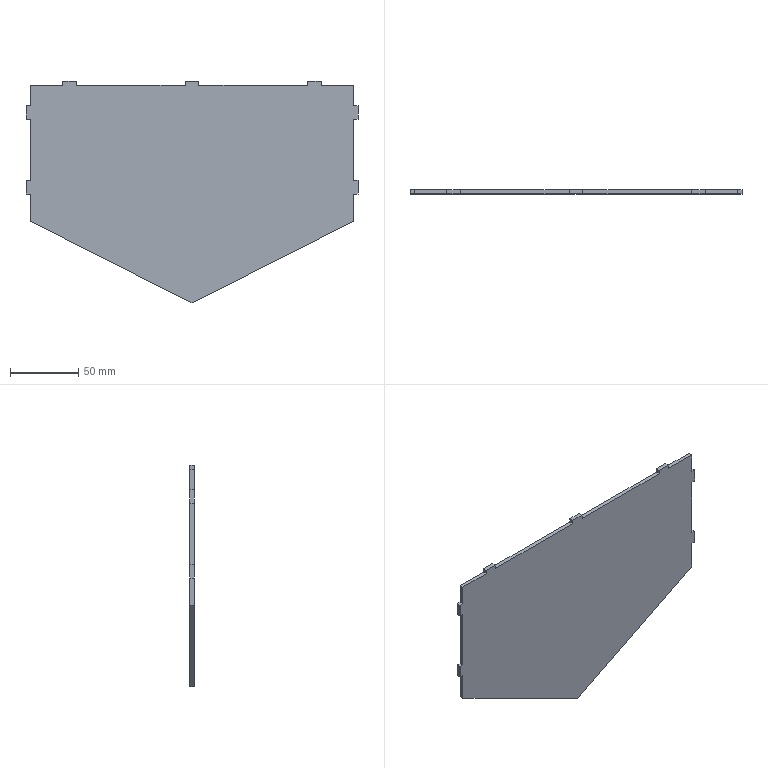Part | SolidWorks | features Extrusion 1, ICE 1 | 1 solid | 35 faces | box 244 x 3 x 163 mm | volume 93450 mm3 | plane 35
STEP:
#1=CARTESIAN_POINT('',(5.,3.,50.));
#2=VERTEX_POINT('',#1);
#3=CARTESIAN_POINT('',(85.,3.,50.));
#4=VERTEX_POINT('',#3);
#5=CARTESIAN_POINT('',(-119.,3.,50.));
#6=DIRECTION('',(1.,0.,0.));
#7=VECTOR('',#6,1000.);
#8=LINE('',#5,#7);
#9=EDGE_CURVE('',#2,#4,#8,.T.);
#10=ORIENTED_EDGE('',*,*,#9,.F.);
#11=CARTESIAN_POINT('',(5.,0.,50.));
#12=VERTEX_POINT('',#11);
#13=CARTESIAN_POINT('',(5.,-10.44,50.));
#14=DIRECTION('',(0.,1.,0.));
#15=VECTOR('',#14,1000.);
#16=LINE('',#13,#15);
#17=EDGE_CURVE('',#12,#2,#16,.T.);
#18=ORIENTED_EDGE('',*,*,#17,.F.);
#19=CARTESIAN_POINT('',(85.,0.,50.));
#20=VERTEX_POINT('',#19);
#21=CARTESIAN_POINT('',(-119.,0.,50.));
#22=DIRECTION('',(1.,0.,0.));
#23=VECTOR('',#22,1000.);
#24=LINE('',#21,#23);
#25=EDGE_CURVE('',#12,#20,#24,.T.);
#26=ORIENTED_EDGE('',*,*,#25,.T.);
#27=CARTESIAN_POINT('',(85.,-10.44,50.));
#28=DIRECTION('',(0.,1.,0.));
#29=VECTOR('',#28,1000.);
#30=LINE('',#27,#29);
#31=EDGE_CURVE('',#20,#4,#30,.T.);
#32=ORIENTED_EDGE('',*,*,#31,.T.);
#33=EDGE_LOOP('',(#10,#18,#26,#32));
#34=FACE_OUTER_BOUND('',#33,.T.);
#35=CARTESIAN_POINT('',(-119.,3.,50.));
#36=DIRECTION('',(0.,0.,-1.));
#37=DIRECTION('',(-1.,0.,0.));
#38=AXIS2_PLACEMENT_3D('',#35,#36,#37);
#39=PLANE('',#38);
#40=ADVANCED_FACE('',(#34),#39,.F.);
#41=CARTESIAN_POINT('',(-85.,0.,50.));
#42=VERTEX_POINT('',#41);
#43=CARTESIAN_POINT('',(-5.,0.,50.));
#44=VERTEX_POINT('',#43);
#45=CARTESIAN_POINT('',(-119.,0.,50.));
#46=DIRECTION('',(1.,0.,0.));
#47=VECTOR('',#46,1000.);
#48=LINE('',#45,#47);
#49=EDGE_CURVE('',#42,#44,#48,.T.);
#50=ORIENTED_EDGE('',*,*,#49,.T.);
#51=CARTESIAN_POINT('',(-5.,3.,50.));
#52=VERTEX_POINT('',#51);
#53=CARTESIAN_POINT('',(-5.,-10.44,50.));
#54=DIRECTION('',(0.,1.,0.));
#55=VECTOR('',#54,1000.);
#56=LINE('',#53,#55);
#57=EDGE_CURVE('',#44,#52,#56,.T.);
#58=ORIENTED_EDGE('',*,*,#57,.T.);
#59=CARTESIAN_POINT('',(-85.,3.,50.));
#60=VERTEX_POINT('',#59);
#61=CARTESIAN_POINT('',(-119.,3.,50.));
#62=DIRECTION('',(1.,0.,0.));
#63=VECTOR('',#62,1000.);
#64=LINE('',#61,#63);
#65=EDGE_CURVE('',#60,#52,#64,.T.);
#66=ORIENTED_EDGE('',*,*,#65,.F.);
#67=CARTESIAN_POINT('',(-85.,-10.44,50.));
#68=DIRECTION('',(0.,1.,0.));
#69=VECTOR('',#68,1000.);
#70=LINE('',#67,#69);
#71=EDGE_CURVE('',#42,#60,#70,.T.);
#72=ORIENTED_EDGE('',*,*,#71,.F.);
#73=EDGE_LOOP('',(#50,#58,#66,#72));
#74=FACE_OUTER_BOUND('',#73,.T.);
#75=CARTESIAN_POINT('',(-119.,3.,50.));
#76=DIRECTION('',(0.,0.,-1.));
#77=DIRECTION('',(-1.,0.,0.));
#78=AXIS2_PLACEMENT_3D('',#75,#76,#77);
#79=PLANE('',#78);
#80=ADVANCED_FACE('',(#74),#79,.F.);
#81=CARTESIAN_POINT('',(95.,0.,50.));
#82=VERTEX_POINT('',#81);
#83=CARTESIAN_POINT('',(95.,3.,50.));
#84=VERTEX_POINT('',#83);
#85=CARTESIAN_POINT('',(95.,-10.44,50.));
#86=DIRECTION('',(0.,1.,0.));
#87=VECTOR('',#86,1000.);
#88=LINE('',#85,#87);
#89=EDGE_CURVE('',#82,#84,#88,.T.);
#90=ORIENTED_EDGE('',*,*,#89,.F.);
#91=CARTESIAN_POINT('',(119.,0.,50.));
#92=VERTEX_POINT('',#91);
#93=CARTESIAN_POINT('',(-119.,0.,50.));
#94=DIRECTION('',(1.,0.,0.));
#95=VECTOR('',#94,1000.);
#96=LINE('',#93,#95);
#97=EDGE_CURVE('',#82,#92,#96,.T.);
#98=ORIENTED_EDGE('',*,*,#97,.T.);
#99=CARTESIAN_POINT('',(119.,3.,50.));
#100=VERTEX_POINT('',#99);
#101=CARTESIAN_POINT('',(119.,3.,50.));
#102=DIRECTION('',(0.,-1.,0.));
#103=VECTOR('',#102,1000.);
#104=LINE('',#101,#103);
#105=EDGE_CURVE('',#100,#92,#104,.T.);
#106=ORIENTED_EDGE('',*,*,#105,.F.);
#107=CARTESIAN_POINT('',(-119.,3.,50.));
#108=DIRECTION('',(1.,0.,0.));
#109=VECTOR('',#108,1000.);
#110=LINE('',#107,#109);
#111=EDGE_CURVE('',#84,#100,#110,.T.);
#112=ORIENTED_EDGE('',*,*,#111,.F.);
#113=EDGE_LOOP('',(#90,#98,#106,#112));
#114=FACE_OUTER_BOUND('',#113,.T.);
#115=CARTESIAN_POINT('',(-119.,3.,50.));
#116=DIRECTION('',(0.,0.,-1.));
#117=DIRECTION('',(-1.,0.,0.));
#118=AXIS2_PLACEMENT_3D('',#115,#116,#117);
#119=PLANE('',#118);
#120=ADVANCED_FACE('',(#114),#119,.F.);
#121=CARTESIAN_POINT('',(-119.,0.,-50.));
#122=VERTEX_POINT('',#121);
#123=CARTESIAN_POINT('',(-119.,0.,-30.));
#124=VERTEX_POINT('',#123);
#125=CARTESIAN_POINT('',(-119.,0.,50.));
#126=DIRECTION('',(0.,0.,1.));
#127=VECTOR('',#126,1000.);
#128=LINE('',#125,#127);
#129=EDGE_CURVE('',#122,#124,#128,.T.);
#130=ORIENTED_EDGE('',*,*,#129,.T.);
#131=CARTESIAN_POINT('',(-119.,3.,-30.));
#132=VERTEX_POINT('',#131);
#133=CARTESIAN_POINT('',(-119.,-10.44,-30.));
#134=DIRECTION('',(0.,1.,0.));
#135=VECTOR('',#134,1000.);
#136=LINE('',#133,#135);
#137=EDGE_CURVE('',#124,#132,#136,.T.);
#138=ORIENTED_EDGE('',*,*,#137,.T.);
#139=CARTESIAN_POINT('',(-119.,3.,-50.));
#140=VERTEX_POINT('',#139);
#141=CARTESIAN_POINT('',(-119.,3.,50.));
#142=DIRECTION('',(0.,0.,1.));
#143=VECTOR('',#142,1000.);
#144=LINE('',#141,#143);
#145=EDGE_CURVE('',#140,#132,#144,.T.);
#146=ORIENTED_EDGE('',*,*,#145,.F.);
#147=CARTESIAN_POINT('',(-119.,3.,-50.));
#148=DIRECTION('',(0.,-1.,0.));
#149=VECTOR('',#148,1000.);
#150=LINE('',#147,#149);
#151=EDGE_CURVE('',#140,#122,#150,.T.);
#152=ORIENTED_EDGE('',*,*,#151,.T.);
#153=EDGE_LOOP('',(#130,#138,#146,#152));
#154=FACE_OUTER_BOUND('',#153,.T.);
#155=CARTESIAN_POINT('',(-119.,3.,50.));
#156=DIRECTION('',(1.,0.,0.));
#157=DIRECTION('',(0.,0.,-1.));
#158=AXIS2_PLACEMENT_3D('',#155,#156,#157);
#159=PLANE('',#158);
#160=ADVANCED_FACE('',(#154),#159,.F.);
#161=CARTESIAN_POINT('',(-119.,0.,35.));
#162=VERTEX_POINT('',#161);
#163=CARTESIAN_POINT('',(-119.,3.,35.));
#164=VERTEX_POINT('',#163);
#165=CARTESIAN_POINT('',(-119.,-10.44,35.));
#166=DIRECTION('',(0.,1.,0.));
#167=VECTOR('',#166,1000.);
#168=LINE('',#165,#167);
#169=EDGE_CURVE('',#162,#164,#168,.T.);
#170=ORIENTED_EDGE('',*,*,#169,.F.);
#171=CARTESIAN_POINT('',(-119.,0.,50.));
#172=VERTEX_POINT('',#171);
#173=CARTESIAN_POINT('',(-119.,0.,50.));
#174=DIRECTION('',(0.,0.,1.));
#175=VECTOR('',#174,1000.);
#176=LINE('',#173,#175);
#177=EDGE_CURVE('',#162,#172,#176,.T.);
#178=ORIENTED_EDGE('',*,*,#177,.T.);
#179=CARTESIAN_POINT('',(-119.,3.,50.));
#180=VERTEX_POINT('',#179);
#181=CARTESIAN_POINT('',(-119.,3.,50.));
#182=DIRECTION('',(0.,-1.,0.));
#183=VECTOR('',#182,1000.);
#184=LINE('',#181,#183);
#185=EDGE_CURVE('',#180,#172,#184,.T.);
#186=ORIENTED_EDGE('',*,*,#185,.F.);
#187=CARTESIAN_POINT('',(-119.,3.,50.));
#188=DIRECTION('',(0.,0.,1.));
#189=VECTOR('',#188,1000.);
#190=LINE('',#187,#189);
#191=EDGE_CURVE('',#164,#180,#190,.T.);
#192=ORIENTED_EDGE('',*,*,#191,.F.);
#193=EDGE_LOOP('',(#170,#178,#186,#192));
#194=FACE_OUTER_BOUND('',#193,.T.);
#195=CARTESIAN_POINT('',(-119.,3.,50.));
#196=DIRECTION('',(1.,0.,0.));
#197=DIRECTION('',(0.,0.,-1.));
#198=AXIS2_PLACEMENT_3D('',#195,#196,#197);
#199=PLANE('',#198);
#200=ADVANCED_FACE('',(#194),#199,.F.);
#201=CARTESIAN_POINT('',(119.,3.,25.));
#202=VERTEX_POINT('',#201);
#203=CARTESIAN_POINT('',(119.,3.,-20.));
#204=VERTEX_POINT('',#203);
#205=CARTESIAN_POINT('',(119.,3.,50.));
#206=DIRECTION('',(0.,0.,-1.));
#207=VECTOR('',#206,1000.);
#208=LINE('',#205,#207);
#209=EDGE_CURVE('',#202,#204,#208,.T.);
#210=ORIENTED_EDGE('',*,*,#209,.F.);
#211=CARTESIAN_POINT('',(119.,0.,25.));
#212=VERTEX_POINT('',#211);
#213=CARTESIAN_POINT('',(119.,-10.44,25.));
#214=DIRECTION('',(0.,1.,0.));
#215=VECTOR('',#214,1000.);
#216=LINE('',#213,#215);
#217=EDGE_CURVE('',#212,#202,#216,.T.);
#218=ORIENTED_EDGE('',*,*,#217,.F.);
#219=CARTESIAN_POINT('',(119.,0.,-20.));
#220=VERTEX_POINT('',#219);
#221=CARTESIAN_POINT('',(119.,0.,50.));
#222=DIRECTION('',(0.,0.,-1.));
#223=VECTOR('',#222,1000.);
#224=LINE('',#221,#223);
#225=EDGE_CURVE('',#212,#220,#224,.T.);
#226=ORIENTED_EDGE('',*,*,#225,.T.);
#227=CARTESIAN_POINT('',(119.,-10.44,-20.));
#228=DIRECTION('',(0.,1.,0.));
#229=VECTOR('',#228,1000.);
#230=LINE('',#227,#229);
#231=EDGE_CURVE('',#220,#204,#230,.T.);
#232=ORIENTED_EDGE('',*,*,#231,.T.);
#233=EDGE_LOOP('',(#210,#218,#226,#232));
#234=FACE_OUTER_BOUND('',#233,.T.);
#235=CARTESIAN_POINT('',(119.,3.,50.));
#236=DIRECTION('',(-1.,0.,0.));
#237=DIRECTION('',(0.,0.,1.));
#238=AXIS2_PLACEMENT_3D('',#235,#236,#237);
#239=PLANE('',#238);
#240=ADVANCED_FACE('',(#234),#239,.F.);
#241=CARTESIAN_POINT('',(119.,0.,-30.));
#242=VERTEX_POINT('',#241);
#243=CARTESIAN_POINT('',(119.,3.,-30.));
#244=VERTEX_POINT('',#243);
#245=CARTESIAN_POINT('',(119.,-10.44,-30.));
#246=DIRECTION('',(0.,1.,0.));
#247=VECTOR('',#246,1000.);
#248=LINE('',#245,#247);
#249=EDGE_CURVE('',#242,#244,#248,.T.);
#250=ORIENTED_EDGE('',*,*,#249,.F.);
#251=CARTESIAN_POINT('',(119.,0.,-50.));
#252=VERTEX_POINT('',#251);
#253=CARTESIAN_POINT('',(119.,0.,50.));
#254=DIRECTION('',(0.,0.,-1.));
#255=VECTOR('',#254,1000.);
#256=LINE('',#253,#255);
#257=EDGE_CURVE('',#242,#252,#256,.T.);
#258=ORIENTED_EDGE('',*,*,#257,.T.);
#259=CARTESIAN_POINT('',(119.,3.,-50.));
#260=VERTEX_POINT('',#259);
#261=CARTESIAN_POINT('',(119.,3.,-50.));
#262=DIRECTION('',(0.,-1.,0.));
#263=VECTOR('',#262,1000.);
#264=LINE('',#261,#263);
#265=EDGE_CURVE('',#260,#252,#264,.T.);
#266=ORIENTED_EDGE('',*,*,#265,.F.);
#267=CARTESIAN_POINT('',(119.,3.,50.));
#268=DIRECTION('',(0.,0.,-1.));
#269=VECTOR('',#268,1000.);
#270=LINE('',#267,#269);
#271=EDGE_CURVE('',#244,#260,#270,.T.);
#272=ORIENTED_EDGE('',*,*,#271,.F.);
#273=EDGE_LOOP('',(#250,#258,#266,#272));
#274=FACE_OUTER_BOUND('',#273,.T.);
#275=CARTESIAN_POINT('',(119.,3.,50.));
#276=DIRECTION('',(-1.,0.,0.));
#277=DIRECTION('',(0.,0.,1.));
#278=AXIS2_PLACEMENT_3D('',#275,#276,#277);
#279=PLANE('',#278);
#280=ADVANCED_FACE('',(#274),#279,.F.);
#281=CARTESIAN_POINT('',(0.,0.,-110.));
#282=VERTEX_POINT('',#281);
#283=CARTESIAN_POINT('',(0.,0.,-110.));
#284=DIRECTION('',(-0.8929,0.,-0.4502));
#285=VECTOR('',#284,1000.);
#286=LINE('',#283,#285);
#287=EDGE_CURVE('',#252,#282,#286,.T.);
#288=ORIENTED_EDGE('',*,*,#287,.T.);
#289=CARTESIAN_POINT('',(0.,3.,-110.));
#290=VERTEX_POINT('',#289);
#291=CARTESIAN_POINT('',(0.,3.,-110.));
#292=DIRECTION('',(0.,-1.,0.));
#293=VECTOR('',#292,1000.);
#294=LINE('',#291,#293);
#295=EDGE_CURVE('',#290,#282,#294,.T.);
#296=ORIENTED_EDGE('',*,*,#295,.F.);
#297=CARTESIAN_POINT('',(0.,3.,-110.));
#298=DIRECTION('',(-0.8929,0.,-0.4502));
#299=VECTOR('',#298,1000.);
#300=LINE('',#297,#299);
#301=EDGE_CURVE('',#260,#290,#300,.T.);
#302=ORIENTED_EDGE('',*,*,#301,.F.);
#303=ORIENTED_EDGE('',*,*,#265,.T.);
#304=EDGE_LOOP('',(#288,#296,#302,#303));
#305=FACE_OUTER_BOUND('',#304,.T.);
#306=CARTESIAN_POINT('',(0.,3.,-110.));
#307=DIRECTION('',(-0.4502,0.,0.8929));
#308=DIRECTION('',(0.8929,0.,0.4502));
#309=AXIS2_PLACEMENT_3D('',#306,#307,#308);
#310=PLANE('',#309);
#311=ADVANCED_FACE('',(#305),#310,.F.);
#312=CARTESIAN_POINT('',(-119.,0.,-50.));
#313=DIRECTION('',(-0.8929,0.,0.4502));
#314=VECTOR('',#313,1000.);
#315=LINE('',#312,#314);
#316=EDGE_CURVE('',#282,#122,#315,.T.);
#317=ORIENTED_EDGE('',*,*,#316,.T.);
#318=ORIENTED_EDGE('',*,*,#151,.F.);
#319=CARTESIAN_POINT('',(-119.,3.,-50.));
#320=DIRECTION('',(-0.8929,0.,0.4502));
#321=VECTOR('',#320,1000.);
#322=LINE('',#319,#321);
#323=EDGE_CURVE('',#290,#140,#322,.T.);
#324=ORIENTED_EDGE('',*,*,#323,.F.);
#325=ORIENTED_EDGE('',*,*,#295,.T.);
#326=EDGE_LOOP('',(#317,#318,#324,#325));
#327=FACE_OUTER_BOUND('',#326,.T.);
#328=CARTESIAN_POINT('',(-119.,3.,-50.));
#329=DIRECTION('',(0.4502,0.,0.8929));
#330=DIRECTION('',(0.8929,0.,-0.4502));
#331=AXIS2_PLACEMENT_3D('',#328,#329,#330);
#332=PLANE('',#331);
#333=ADVANCED_FACE('',(#327),#332,.F.);
#334=CARTESIAN_POINT('',(-119.,3.,-20.));
#335=VERTEX_POINT('',#334);
#336=CARTESIAN_POINT('',(-119.,3.,25.));
#337=VERTEX_POINT('',#336);
#338=CARTESIAN_POINT('',(-119.,3.,50.));
#339=DIRECTION('',(0.,0.,1.));
#340=VECTOR('',#339,1000.);
#341=LINE('',#338,#340);
#342=EDGE_CURVE('',#335,#337,#341,.T.);
#343=ORIENTED_EDGE('',*,*,#342,.F.);
#344=CARTESIAN_POINT('',(-119.,0.,-20.));
#345=VERTEX_POINT('',#344);
#346=CARTESIAN_POINT('',(-119.,-10.44,-20.));
#347=DIRECTION('',(0.,1.,0.));
#348=VECTOR('',#347,1000.);
#349=LINE('',#346,#348);
#350=EDGE_CURVE('',#345,#335,#349,.T.);
#351=ORIENTED_EDGE('',*,*,#350,.F.);
#352=CARTESIAN_POINT('',(-119.,0.,25.));
#353=VERTEX_POINT('',#352);
#354=CARTESIAN_POINT('',(-119.,0.,50.));
#355=DIRECTION('',(0.,0.,1.));
#356=VECTOR('',#355,1000.);
#357=LINE('',#354,#356);
#358=EDGE_CURVE('',#345,#353,#357,.T.);
#359=ORIENTED_EDGE('',*,*,#358,.T.);
#360=CARTESIAN_POINT('',(-119.,-10.44,25.));
#361=DIRECTION('',(0.,1.,0.));
#362=VECTOR('',#361,1000.);
#363=LINE('',#360,#362);
#364=EDGE_CURVE('',#353,#337,#363,.T.);
#365=ORIENTED_EDGE('',*,*,#364,.T.);
#366=EDGE_LOOP('',(#343,#351,#359,#365));
#367=FACE_OUTER_BOUND('',#366,.T.);
#368=CARTESIAN_POINT('',(-119.,3.,50.));
#369=DIRECTION('',(1.,0.,0.));
#370=DIRECTION('',(0.,0.,-1.));
#371=AXIS2_PLACEMENT_3D('',#368,#369,#370);
#372=PLANE('',#371);
#373=ADVANCED_FACE('',(#367),#372,.F.);
#374=CARTESIAN_POINT('',(-95.,0.,50.));
#375=VERTEX_POINT('',#374);
#376=CARTESIAN_POINT('',(-119.,0.,50.));
#377=DIRECTION('',(1.,0.,0.));
#378=VECTOR('',#377,1000.);
#379=LINE('',#376,#378);
#380=EDGE_CURVE('',#172,#375,#379,.T.);
#381=ORIENTED_EDGE('',*,*,#380,.T.);
#382=CARTESIAN_POINT('',(-95.,3.,50.));
#383=VERTEX_POINT('',#382);
#384=CARTESIAN_POINT('',(-95.,-10.44,50.));
#385=DIRECTION('',(0.,1.,0.));
#386=VECTOR('',#385,1000.);
#387=LINE('',#384,#386);
#388=EDGE_CURVE('',#375,#383,#387,.T.);
#389=ORIENTED_EDGE('',*,*,#388,.T.);
#390=CARTESIAN_POINT('',(-119.,3.,50.));
#391=DIRECTION('',(1.,0.,0.));
#392=VECTOR('',#391,1000.);
#393=LINE('',#390,#392);
#394=EDGE_CURVE('',#180,#383,#393,.T.);
#395=ORIENTED_EDGE('',*,*,#394,.F.);
#396=ORIENTED_EDGE('',*,*,#185,.T.);
#397=EDGE_LOOP('',(#381,#389,#395,#396));
#398=FACE_OUTER_BOUND('',#397,.T.);
#399=CARTESIAN_POINT('',(-119.,3.,50.));
#400=DIRECTION('',(0.,0.,-1.));
#401=DIRECTION('',(-1.,0.,0.));
#402=AXIS2_PLACEMENT_3D('',#399,#400,#401);
#403=PLANE('',#402);
#404=ADVANCED_FACE('',(#398),#403,.F.);
#405=CARTESIAN_POINT('',(119.,0.,35.));
#406=VERTEX_POINT('',#405);
#407=CARTESIAN_POINT('',(119.,0.,50.));
#408=DIRECTION('',(0.,0.,-1.));
#409=VECTOR('',#408,1000.);
#410=LINE('',#407,#409);
#411=EDGE_CURVE('',#92,#406,#410,.T.);
#412=ORIENTED_EDGE('',*,*,#411,.T.);
#413=CARTESIAN_POINT('',(119.,3.,35.));
#414=VERTEX_POINT('',#413);
#415=CARTESIAN_POINT('',(119.,-10.44,35.));
#416=DIRECTION('',(0.,1.,0.));
#417=VECTOR('',#416,1000.);
#418=LINE('',#415,#417);
#419=EDGE_CURVE('',#406,#414,#418,.T.);
#420=ORIENTED_EDGE('',*,*,#419,.T.);
#421=CARTESIAN_POINT('',(119.,3.,50.));
#422=DIRECTION('',(0.,0.,-1.));
#423=VECTOR('',#422,1000.);
#424=LINE('',#421,#423);
#425=EDGE_CURVE('',#100,#414,#424,.T.);
#426=ORIENTED_EDGE('',*,*,#425,.F.);
#427=ORIENTED_EDGE('',*,*,#105,.T.);
#428=EDGE_LOOP('',(#412,#420,#426,#427));
#429=FACE_OUTER_BOUND('',#428,.T.);
#430=CARTESIAN_POINT('',(119.,3.,50.));
#431=DIRECTION('',(-1.,0.,0.));
#432=DIRECTION('',(0.,0.,1.));
#433=AXIS2_PLACEMENT_3D('',#430,#431,#432);
#434=PLANE('',#433);
#435=ADVANCED_FACE('',(#429),#434,.F.);
#436=ORIENTED_EDGE('',*,*,#301,.T.);
#437=ORIENTED_EDGE('',*,*,#323,.T.);
#438=ORIENTED_EDGE('',*,*,#145,.T.);
#439=CARTESIAN_POINT('',(-122.,3.,-30.));
#440=VERTEX_POINT('',#439);
#441=CARTESIAN_POINT('',(-119.,3.,-30.));
#442=DIRECTION('',(-1.,0.,0.));
#443=VECTOR('',#442,1000.);
#444=LINE('',#441,#443);
#445=EDGE_CURVE('',#132,#440,#444,.T.);
#446=ORIENTED_EDGE('',*,*,#445,.T.);
#447=CARTESIAN_POINT('',(-122.,3.,-20.));
#448=VERTEX_POINT('',#447);
#449=CARTESIAN_POINT('',(-122.,3.,-30.));
#450=DIRECTION('',(0.,0.,1.));
#451=VECTOR('',#450,1000.);
#452=LINE('',#449,#451);
#453=EDGE_CURVE('',#440,#448,#452,.T.);
#454=ORIENTED_EDGE('',*,*,#453,.T.);
#455=CARTESIAN_POINT('',(-119.,3.,-20.));
#456=DIRECTION('',(1.,0.,0.));
#457=VECTOR('',#456,1000.);
#458=LINE('',#455,#457);
#459=EDGE_CURVE('',#448,#335,#458,.T.);
#460=ORIENTED_EDGE('',*,*,#459,.T.);
#461=ORIENTED_EDGE('',*,*,#342,.T.);
#462=CARTESIAN_POINT('',(-122.,3.,25.));
#463=VERTEX_POINT('',#462);
#464=CARTESIAN_POINT('',(-119.,3.,25.));
#465=DIRECTION('',(-1.,0.,0.));
#466=VECTOR('',#465,1000.);
#467=LINE('',#464,#466);
#468=EDGE_CURVE('',#337,#463,#467,.T.);
#469=ORIENTED_EDGE('',*,*,#468,.T.);
#470=CARTESIAN_POINT('',(-122.,3.,35.));
#471=VERTEX_POINT('',#470);
#472=CARTESIAN_POINT('',(-122.,3.,35.));
#473=DIRECTION('',(0.,0.,1.));
#474=VECTOR('',#473,1000.);
#475=LINE('',#472,#474);
#476=EDGE_CURVE('',#463,#471,#475,.T.);
#477=ORIENTED_EDGE('',*,*,#476,.T.);
#478=CARTESIAN_POINT('',(-119.,3.,35.));
#479=DIRECTION('',(1.,0.,0.));
#480=VECTOR('',#479,1000.);
#481=LINE('',#478,#480);
#482=EDGE_CURVE('',#471,#164,#481,.T.);
#483=ORIENTED_EDGE('',*,*,#482,.T.);
#484=ORIENTED_EDGE('',*,*,#191,.T.);
#485=ORIENTED_EDGE('',*,*,#394,.T.);
#486=CARTESIAN_POINT('',(-95.,3.,53.));
#487=VERTEX_POINT('',#486);
#488=CARTESIAN_POINT('',(-95.,3.,50.));
#489=DIRECTION('',(0.,0.,1.));
#490=VECTOR('',#489,1000.);
#491=LINE('',#488,#490);
#492=EDGE_CURVE('',#383,#487,#491,.T.);
#493=ORIENTED_EDGE('',*,*,#492,.T.);
#494=CARTESIAN_POINT('',(-85.,3.,53.));
#495=VERTEX_POINT('',#494);
#496=CARTESIAN_POINT('',(-85.,3.,53.));
#497=DIRECTION('',(1.,0.,0.));
#498=VECTOR('',#497,1000.);
#499=LINE('',#496,#498);
#500=EDGE_CURVE('',#487,#495,#499,.T.);
#501=ORIENTED_EDGE('',*,*,#500,.T.);
#502=CARTESIAN_POINT('',(-85.,3.,50.));
#503=DIRECTION('',(0.,0.,-1.));
#504=VECTOR('',#503,1000.);
#505=LINE('',#502,#504);
#506=EDGE_CURVE('',#495,#60,#505,.T.);
#507=ORIENTED_EDGE('',*,*,#506,.T.);
#508=ORIENTED_EDGE('',*,*,#65,.T.);
#509=CARTESIAN_POINT('',(-5.,3.,53.));
#510=VERTEX_POINT('',#509);
#511=CARTESIAN_POINT('',(-5.,3.,53.));
#512=DIRECTION('',(0.,0.,1.));
#513=VECTOR('',#512,1000.);
#514=LINE('',#511,#513);
#515=EDGE_CURVE('',#52,#510,#514,.T.);
#516=ORIENTED_EDGE('',*,*,#515,.T.);
#517=CARTESIAN_POINT('',(5.,3.,53.));
#518=VERTEX_POINT('',#517);
#519=CARTESIAN_POINT('',(-5.,3.,53.));
#520=DIRECTION('',(1.,0.,0.));
#521=VECTOR('',#520,1000.);
#522=LINE('',#519,#521);
#523=EDGE_CURVE('',#510,#518,#522,.T.);
#524=ORIENTED_EDGE('',*,*,#523,.T.);
#525=CARTESIAN_POINT('',(5.,3.,53.));
#526=DIRECTION('',(0.,0.,-1.));
#527=VECTOR('',#526,1000.);
#528=LINE('',#525,#527);
#529=EDGE_CURVE('',#518,#2,#528,.T.);
#530=ORIENTED_EDGE('',*,*,#529,.T.);
#531=ORIENTED_EDGE('',*,*,#9,.T.);
#532=CARTESIAN_POINT('',(85.,3.,53.));
#533=VERTEX_POINT('',#532);
#534=CARTESIAN_POINT('',(85.,3.,50.));
#535=DIRECTION('',(0.,0.,1.));
#536=VECTOR('',#535,1000.);
#537=LINE('',#534,#536);
#538=EDGE_CURVE('',#4,#533,#537,.T.);
#539=ORIENTED_EDGE('',*,*,#538,.T.);
#540=CARTESIAN_POINT('',(95.,3.,53.));
#541=VERTEX_POINT('',#540);
#542=CARTESIAN_POINT('',(85.,3.,53.));
#543=DIRECTION('',(1.,0.,0.));
#544=VECTOR('',#543,1000.);
#545=LINE('',#542,#544);
#546=EDGE_CURVE('',#533,#541,#545,.T.);
#547=ORIENTED_EDGE('',*,*,#546,.T.);
#548=CARTESIAN_POINT('',(95.,3.,50.));
#549=DIRECTION('',(0.,0.,-1.));
#550=VECTOR('',#549,1000.);
#551=LINE('',#548,#550);
#552=EDGE_CURVE('',#541,#84,#551,.T.);
#553=ORIENTED_EDGE('',*,*,#552,.T.);
#554=ORIENTED_EDGE('',*,*,#111,.T.);
#555=ORIENTED_EDGE('',*,*,#425,.T.);
#556=CARTESIAN_POINT('',(122.,3.,35.));
#557=VERTEX_POINT('',#556);
#558=CARTESIAN_POINT('',(119.,3.,35.));
#559=DIRECTION('',(1.,0.,0.));
#560=VECTOR('',#559,1000.);
#561=LINE('',#558,#560);
#562=EDGE_CURVE('',#414,#557,#561,.T.);
#563=ORIENTED_EDGE('',*,*,#562,.T.);
#564=CARTESIAN_POINT('',(122.,3.,25.));
#565=VERTEX_POINT('',#564);
#566=CARTESIAN_POINT('',(122.,3.,35.));
#567=DIRECTION('',(0.,0.,-1.));
#568=VECTOR('',#567,1000.);
#569=LINE('',#566,#568);
#570=EDGE_CURVE('',#557,#565,#569,.T.);
#571=ORIENTED_EDGE('',*,*,#570,.T.);
#572=CARTESIAN_POINT('',(119.,3.,25.));
#573=DIRECTION('',(-1.,0.,0.));
#574=VECTOR('',#573,1000.);
#575=LINE('',#572,#574);
#576=EDGE_CURVE('',#565,#202,#575,.T.);
#577=ORIENTED_EDGE('',*,*,#576,.T.);
#578=ORIENTED_EDGE('',*,*,#209,.T.);
#579=CARTESIAN_POINT('',(122.,3.,-20.));
#580=VERTEX_POINT('',#579);
#581=CARTESIAN_POINT('',(119.,3.,-20.));
#582=DIRECTION('',(1.,0.,0.));
#583=VECTOR('',#582,1000.);
#584=LINE('',#581,#583);
#585=EDGE_CURVE('',#204,#580,#584,.T.);
#586=ORIENTED_EDGE('',*,*,#585,.T.);
#587=CARTESIAN_POINT('',(122.,3.,-30.));
#588=VERTEX_POINT('',#587);
#589=CARTESIAN_POINT('',(122.,3.,-30.));
#590=DIRECTION('',(0.,0.,-1.));
#591=VECTOR('',#590,1000.);
#592=LINE('',#589,#591);
#593=EDGE_CURVE('',#580,#588,#592,.T.);
#594=ORIENTED_EDGE('',*,*,#593,.T.);
#595=CARTESIAN_POINT('',(119.,3.,-30.));
#596=DIRECTION('',(-1.,0.,0.));
#597=VECTOR('',#596,1000.);
#598=LINE('',#595,#597);
#599=EDGE_CURVE('',#588,#244,#598,.T.);
#600=ORIENTED_EDGE('',*,*,#599,.T.);
#601=ORIENTED_EDGE('',*,*,#271,.T.);
#602=EDGE_LOOP('',(#436,#437,#438,#446,#454,#460,#461,#469,#477,#483,#484,#485,#493,#501,#507,#508,#516,#524,#530,#531,#539,#547,#553,#554,#555,#563,#571,#577,#578,#586,#594,#600,#601));
#603=FACE_OUTER_BOUND('',#602,.T.);
#604=CARTESIAN_POINT('',(0.,3.,0.));
#605=DIRECTION('',(0.,1.,0.));
#606=DIRECTION('',(0.,0.,1.));
#607=AXIS2_PLACEMENT_3D('',#604,#605,#606);
#608=PLANE('',#607);
#609=ADVANCED_FACE('',(#603),#608,.T.);
#610=ORIENTED_EDGE('',*,*,#287,.F.);
#611=ORIENTED_EDGE('',*,*,#257,.F.);
#612=CARTESIAN_POINT('',(122.,0.,-30.));
#613=VERTEX_POINT('',#612);
#614=CARTESIAN_POINT('',(119.,0.,-30.));
#615=DIRECTION('',(1.,0.,0.));
#616=VECTOR('',#615,1000.);
#617=LINE('',#614,#616);
#618=EDGE_CURVE('',#242,#613,#617,.T.);
#619=ORIENTED_EDGE('',*,*,#618,.T.);
#620=CARTESIAN_POINT('',(122.,0.,-20.));
#621=VERTEX_POINT('',#620);
#622=CARTESIAN_POINT('',(122.,0.,-30.));
#623=DIRECTION('',(0.,0.,1.));
#624=VECTOR('',#623,1000.);
#625=LINE('',#622,#624);
#626=EDGE_CURVE('',#613,#621,#625,.T.);
#627=ORIENTED_EDGE('',*,*,#626,.T.);
#628=CARTESIAN_POINT('',(119.,0.,-20.));
#629=DIRECTION('',(-1.,0.,0.));
#630=VECTOR('',#629,1000.);
#631=LINE('',#628,#630);
#632=EDGE_CURVE('',#621,#220,#631,.T.);
#633=ORIENTED_EDGE('',*,*,#632,.T.);
#634=ORIENTED_EDGE('',*,*,#225,.F.);
#635=CARTESIAN_POINT('',(122.,0.,25.));
#636=VERTEX_POINT('',#635);
#637=CARTESIAN_POINT('',(119.,0.,25.));
#638=DIRECTION('',(1.,0.,0.));
#639=VECTOR('',#638,1000.);
#640=LINE('',#637,#639);
#641=EDGE_CURVE('',#212,#636,#640,.T.);
#642=ORIENTED_EDGE('',*,*,#641,.T.);
#643=CARTESIAN_POINT('',(122.,0.,35.));
#644=VERTEX_POINT('',#643);
#645=CARTESIAN_POINT('',(122.,0.,35.));
#646=DIRECTION('',(0.,0.,1.));
#647=VECTOR('',#646,1000.);
#648=LINE('',#645,#647);
#649=EDGE_CURVE('',#636,#644,#648,.T.);
#650=ORIENTED_EDGE('',*,*,#649,.T.);
#651=CARTESIAN_POINT('',(119.,0.,35.));
#652=DIRECTION('',(-1.,0.,0.));
#653=VECTOR('',#652,1000.);
#654=LINE('',#651,#653);
#655=EDGE_CURVE('',#644,#406,#654,.T.);
#656=ORIENTED_EDGE('',*,*,#655,.T.);
#657=ORIENTED_EDGE('',*,*,#411,.F.);
#658=ORIENTED_EDGE('',*,*,#97,.F.);
#659=CARTESIAN_POINT('',(95.,0.,53.));
#660=VERTEX_POINT('',#659);
#661=CARTESIAN_POINT('',(95.,0.,50.));
#662=DIRECTION('',(0.,0.,1.));
#663=VECTOR('',#662,1000.);
#664=LINE('',#661,#663);
#665=EDGE_CURVE('',#82,#660,#664,.T.);
#666=ORIENTED_EDGE('',*,*,#665,.T.);
#667=CARTESIAN_POINT('',(85.,0.,53.));
#668=VERTEX_POINT('',#667);
#669=CARTESIAN_POINT('',(85.,0.,53.));
#670=DIRECTION('',(-1.,0.,0.));
#671=VECTOR('',#670,1000.);
#672=LINE('',#669,#671);
#673=EDGE_CURVE('',#660,#668,#672,.T.);
#674=ORIENTED_EDGE('',*,*,#673,.T.);
#675=CARTESIAN_POINT('',(85.,0.,50.));
#676=DIRECTION('',(0.,0.,-1.));
#677=VECTOR('',#676,1000.);
#678=LINE('',#675,#677);
#679=EDGE_CURVE('',#668,#20,#678,.T.);
#680=ORIENTED_EDGE('',*,*,#679,.T.);
#681=ORIENTED_EDGE('',*,*,#25,.F.);
#682=CARTESIAN_POINT('',(5.,0.,53.));
#683=VERTEX_POINT('',#682);
#684=CARTESIAN_POINT('',(5.,0.,53.));
#685=DIRECTION('',(0.,0.,1.));
#686=VECTOR('',#685,1000.);
#687=LINE('',#684,#686);
#688=EDGE_CURVE('',#12,#683,#687,.T.);
#689=ORIENTED_EDGE('',*,*,#688,.T.);
#690=CARTESIAN_POINT('',(-5.,0.,53.));
#691=VERTEX_POINT('',#690);
#692=CARTESIAN_POINT('',(-5.,0.,53.));
#693=DIRECTION('',(-1.,0.,0.));
#694=VECTOR('',#693,1000.);
#695=LINE('',#692,#694);
#696=EDGE_CURVE('',#683,#691,#695,.T.);
#697=ORIENTED_EDGE('',*,*,#696,.T.);
#698=CARTESIAN_POINT('',(-5.,0.,53.));
#699=DIRECTION('',(0.,0.,-1.));
#700=VECTOR('',#699,1000.);
#701=LINE('',#698,#700);
#702=EDGE_CURVE('',#691,#44,#701,.T.);
#703=ORIENTED_EDGE('',*,*,#702,.T.);
#704=ORIENTED_EDGE('',*,*,#49,.F.);
#705=CARTESIAN_POINT('',(-85.,0.,53.));
#706=VERTEX_POINT('',#705);
#707=CARTESIAN_POINT('',(-85.,0.,50.));
#708=DIRECTION('',(0.,0.,1.));
#709=VECTOR('',#708,1000.);
#710=LINE('',#707,#709);
#711=EDGE_CURVE('',#42,#706,#710,.T.);
#712=ORIENTED_EDGE('',*,*,#711,.T.);
#713=CARTESIAN_POINT('',(-95.,0.,53.));
#714=VERTEX_POINT('',#713);
#715=CARTESIAN_POINT('',(-85.,0.,53.));
#716=DIRECTION('',(-1.,0.,0.));
#717=VECTOR('',#716,1000.);
#718=LINE('',#715,#717);
#719=EDGE_CURVE('',#706,#714,#718,.T.);
#720=ORIENTED_EDGE('',*,*,#719,.T.);
#721=CARTESIAN_POINT('',(-95.,0.,50.));
#722=DIRECTION('',(0.,0.,-1.));
#723=VECTOR('',#722,1000.);
#724=LINE('',#721,#723);
#725=EDGE_CURVE('',#714,#375,#724,.T.);
#726=ORIENTED_EDGE('',*,*,#725,.T.);
#727=ORIENTED_EDGE('',*,*,#380,.F.);
#728=ORIENTED_EDGE('',*,*,#177,.F.);
#729=CARTESIAN_POINT('',(-122.,0.,35.));
#730=VERTEX_POINT('',#729);
#731=CARTESIAN_POINT('',(-119.,0.,35.));
#732=DIRECTION('',(-1.,0.,0.));
#733=VECTOR('',#732,1000.);
#734=LINE('',#731,#733);
#735=EDGE_CURVE('',#162,#730,#734,.T.);
#736=ORIENTED_EDGE('',*,*,#735,.T.);
#737=CARTESIAN_POINT('',(-122.,0.,25.));
#738=VERTEX_POINT('',#737);
#739=CARTESIAN_POINT('',(-122.,0.,35.));
#740=DIRECTION('',(0.,0.,-1.));
#741=VECTOR('',#740,1000.);
#742=LINE('',#739,#741);
#743=EDGE_CURVE('',#730,#738,#742,.T.);
#744=ORIENTED_EDGE('',*,*,#743,.T.);
#745=CARTESIAN_POINT('',(-119.,0.,25.));
#746=DIRECTION('',(1.,0.,0.));
#747=VECTOR('',#746,1000.);
#748=LINE('',#745,#747);
#749=EDGE_CURVE('',#738,#353,#748,.T.);
#750=ORIENTED_EDGE('',*,*,#749,.T.);
#751=ORIENTED_EDGE('',*,*,#358,.F.);
#752=CARTESIAN_POINT('',(-122.,0.,-20.));
#753=VERTEX_POINT('',#752);
#754=CARTESIAN_POINT('',(-119.,0.,-20.));
#755=DIRECTION('',(-1.,0.,0.));
#756=VECTOR('',#755,1000.);
#757=LINE('',#754,#756);
#758=EDGE_CURVE('',#345,#753,#757,.T.);
#759=ORIENTED_EDGE('',*,*,#758,.T.);
#760=CARTESIAN_POINT('',(-122.,0.,-30.));
#761=VERTEX_POINT('',#760);
#762=CARTESIAN_POINT('',(-122.,0.,-30.));
#763=DIRECTION('',(0.,0.,-1.));
#764=VECTOR('',#763,1000.);
#765=LINE('',#762,#764);
#766=EDGE_CURVE('',#753,#761,#765,.T.);
#767=ORIENTED_EDGE('',*,*,#766,.T.);
#768=CARTESIAN_POINT('',(-119.,0.,-30.));
#769=DIRECTION('',(1.,0.,0.));
#770=VECTOR('',#769,1000.);
#771=LINE('',#768,#770);
#772=EDGE_CURVE('',#761,#124,#771,.T.);
#773=ORIENTED_EDGE('',*,*,#772,.T.);
#774=ORIENTED_EDGE('',*,*,#129,.F.);
#775=ORIENTED_EDGE('',*,*,#316,.F.);
#776=EDGE_LOOP('',(#610,#611,#619,#627,#633,#634,#642,#650,#656,#657,#658,#666,#674,#680,#681,#689,#697,#703,#704,#712,#720,#726,#727,#728,#736,#744,#750,#751,#759,#767,#773,#774,#775));
#777=FACE_OUTER_BOUND('',#776,.T.);
#778=CARTESIAN_POINT('',(0.,0.,0.));
#779=DIRECTION('',(0.,1.,0.));
#780=DIRECTION('',(0.,0.,1.));
#781=AXIS2_PLACEMENT_3D('',#778,#779,#780);
#782=PLANE('',#781);
#783=ADVANCED_FACE('',(#777),#782,.F.);
#784=ORIENTED_EDGE('',*,*,#618,.F.);
#785=ORIENTED_EDGE('',*,*,#249,.T.);
#786=ORIENTED_EDGE('',*,*,#599,.F.);
#787=CARTESIAN_POINT('',(122.,-10.44,-30.));
#788=DIRECTION('',(0.,1.,0.));
#789=VECTOR('',#788,1000.);
#790=LINE('',#787,#789);
#791=EDGE_CURVE('',#613,#588,#790,.T.);
#792=ORIENTED_EDGE('',*,*,#791,.F.);
#793=EDGE_LOOP('',(#784,#785,#786,#792));
#794=FACE_OUTER_BOUND('',#793,.T.);
#795=CARTESIAN_POINT('',(119.,-10.44,-30.));
#796=DIRECTION('',(0.,0.,-1.));
#797=DIRECTION('',(-1.,0.,0.));
#798=AXIS2_PLACEMENT_3D('',#795,#796,#797);
#799=PLANE('',#798);
#800=ADVANCED_FACE('',(#794),#799,.T.);
#801=ORIENTED_EDGE('',*,*,#626,.F.);
#802=ORIENTED_EDGE('',*,*,#791,.T.);
#803=ORIENTED_EDGE('',*,*,#593,.F.);
#804=CARTESIAN_POINT('',(122.,-10.44,-20.));
#805=DIRECTION('',(0.,1.,0.));
#806=VECTOR('',#805,1000.);
#807=LINE('',#804,#806);
#808=EDGE_CURVE('',#621,#580,#807,.T.);
#809=ORIENTED_EDGE('',*,*,#808,.F.);
#810=EDGE_LOOP('',(#801,#802,#803,#809));
#811=FACE_OUTER_BOUND('',#810,.T.);
#812=CARTESIAN_POINT('',(122.,-10.44,-30.));
#813=DIRECTION('',(1.,0.,0.));
#814=DIRECTION('',(0.,0.,-1.));
#815=AXIS2_PLACEMENT_3D('',#812,#813,#814);
#816=PLANE('',#815);
#817=ADVANCED_FACE('',(#811),#816,.T.);
#818=ORIENTED_EDGE('',*,*,#632,.F.);
#819=ORIENTED_EDGE('',*,*,#808,.T.);
#820=ORIENTED_EDGE('',*,*,#585,.F.);
#821=ORIENTED_EDGE('',*,*,#231,.F.);
#822=EDGE_LOOP('',(#818,#819,#820,#821));
#823=FACE_OUTER_BOUND('',#822,.T.);
#824=CARTESIAN_POINT('',(119.,-10.44,-20.));
#825=DIRECTION('',(0.,0.,1.));
#826=DIRECTION('',(1.,0.,0.));
#827=AXIS2_PLACEMENT_3D('',#824,#825,#826);
#828=PLANE('',#827);
#829=ADVANCED_FACE('',(#823),#828,.T.);
#830=ORIENTED_EDGE('',*,*,#641,.F.);
#831=ORIENTED_EDGE('',*,*,#217,.T.);
#832=ORIENTED_EDGE('',*,*,#576,.F.);
#833=CARTESIAN_POINT('',(122.,-10.44,25.));
#834=DIRECTION('',(0.,1.,0.));
#835=VECTOR('',#834,1000.);
#836=LINE('',#833,#835);
#837=EDGE_CURVE('',#636,#565,#836,.T.);
#838=ORIENTED_EDGE('',*,*,#837,.F.);
#839=EDGE_LOOP('',(#830,#831,#832,#838));
#840=FACE_OUTER_BOUND('',#839,.T.);
#841=CARTESIAN_POINT('',(119.,-10.44,25.));
#842=DIRECTION('',(0.,0.,-1.));
#843=DIRECTION('',(-1.,0.,0.));
#844=AXIS2_PLACEMENT_3D('',#841,#842,#843);
#845=PLANE('',#844);
#846=ADVANCED_FACE('',(#840),#845,.T.);
#847=ORIENTED_EDGE('',*,*,#649,.F.);
#848=ORIENTED_EDGE('',*,*,#837,.T.);
#849=ORIENTED_EDGE('',*,*,#570,.F.);
#850=CARTESIAN_POINT('',(122.,-10.44,35.));
#851=DIRECTION('',(0.,1.,0.));
#852=VECTOR('',#851,1000.);
#853=LINE('',#850,#852);
#854=EDGE_CURVE('',#644,#557,#853,.T.);
#855=ORIENTED_EDGE('',*,*,#854,.F.);
#856=EDGE_LOOP('',(#847,#848,#849,#855));
#857=FACE_OUTER_BOUND('',#856,.T.);
#858=CARTESIAN_POINT('',(122.,-10.44,35.));
#859=DIRECTION('',(1.,0.,0.));
#860=DIRECTION('',(0.,0.,-1.));
#861=AXIS2_PLACEMENT_3D('',#858,#859,#860);
#862=PLANE('',#861);
#863=ADVANCED_FACE('',(#857),#862,.T.);
#864=ORIENTED_EDGE('',*,*,#655,.F.);
#865=ORIENTED_EDGE('',*,*,#854,.T.);
#866=ORIENTED_EDGE('',*,*,#562,.F.);
#867=ORIENTED_EDGE('',*,*,#419,.F.);
#868=EDGE_LOOP('',(#864,#865,#866,#867));
#869=FACE_OUTER_BOUND('',#868,.T.);
#870=CARTESIAN_POINT('',(119.,-10.44,35.));
#871=DIRECTION('',(0.,0.,1.));
#872=DIRECTION('',(1.,0.,0.));
#873=AXIS2_PLACEMENT_3D('',#870,#871,#872);
#874=PLANE('',#873);
#875=ADVANCED_FACE('',(#869),#874,.T.);
#876=ORIENTED_EDGE('',*,*,#735,.F.);
#877=ORIENTED_EDGE('',*,*,#169,.T.);
#878=ORIENTED_EDGE('',*,*,#482,.F.);
#879=CARTESIAN_POINT('',(-122.,-10.44,35.));
#880=DIRECTION('',(0.,1.,0.));
#881=VECTOR('',#880,1000.);
#882=LINE('',#879,#881);
#883=EDGE_CURVE('',#730,#471,#882,.T.);
#884=ORIENTED_EDGE('',*,*,#883,.F.);
#885=EDGE_LOOP('',(#876,#877,#878,#884));
#886=FACE_OUTER_BOUND('',#885,.T.);
#887=CARTESIAN_POINT('',(-119.,-10.44,35.));
#888=DIRECTION('',(0.,0.,1.));
#889=DIRECTION('',(1.,0.,0.));
#890=AXIS2_PLACEMENT_3D('',#887,#888,#889);
#891=PLANE('',#890);
#892=ADVANCED_FACE('',(#886),#891,.T.);
#893=ORIENTED_EDGE('',*,*,#743,.F.);
#894=ORIENTED_EDGE('',*,*,#883,.T.);
#895=ORIENTED_EDGE('',*,*,#476,.F.);
#896=CARTESIAN_POINT('',(-122.,-10.44,25.));
#897=DIRECTION('',(0.,1.,0.));
#898=VECTOR('',#897,1000.);
#899=LINE('',#896,#898);
#900=EDGE_CURVE('',#738,#463,#899,.T.);
#901=ORIENTED_EDGE('',*,*,#900,.F.);
#902=EDGE_LOOP('',(#893,#894,#895,#901));
#903=FACE_OUTER_BOUND('',#902,.T.);
#904=CARTESIAN_POINT('',(-122.,-10.44,35.));
#905=DIRECTION('',(-1.,0.,0.));
#906=DIRECTION('',(0.,0.,1.));
#907=AXIS2_PLACEMENT_3D('',#904,#905,#906);
#908=PLANE('',#907);
#909=ADVANCED_FACE('',(#903),#908,.T.);
#910=ORIENTED_EDGE('',*,*,#749,.F.);
#911=ORIENTED_EDGE('',*,*,#900,.T.);
#912=ORIENTED_EDGE('',*,*,#468,.F.);
#913=ORIENTED_EDGE('',*,*,#364,.F.);
#914=EDGE_LOOP('',(#910,#911,#912,#913));
#915=FACE_OUTER_BOUND('',#914,.T.);
#916=CARTESIAN_POINT('',(-119.,-10.44,25.));
#917=DIRECTION('',(0.,0.,-1.));
#918=DIRECTION('',(-1.,0.,0.));
#919=AXIS2_PLACEMENT_3D('',#916,#917,#918);
#920=PLANE('',#919);
#921=ADVANCED_FACE('',(#915),#920,.T.);
#922=ORIENTED_EDGE('',*,*,#772,.F.);
#923=CARTESIAN_POINT('',(-122.,-10.44,-30.));
#924=DIRECTION('',(0.,1.,0.));
#925=VECTOR('',#924,1000.);
#926=LINE('',#923,#925);
#927=EDGE_CURVE('',#761,#440,#926,.T.);
#928=ORIENTED_EDGE('',*,*,#927,.T.);
#929=ORIENTED_EDGE('',*,*,#445,.F.);
#930=ORIENTED_EDGE('',*,*,#137,.F.);
#931=EDGE_LOOP('',(#922,#928,#929,#930));
#932=FACE_OUTER_BOUND('',#931,.T.);
#933=CARTESIAN_POINT('',(-119.,-10.44,-30.));
#934=DIRECTION('',(0.,0.,-1.));
#935=DIRECTION('',(-1.,0.,0.));
#936=AXIS2_PLACEMENT_3D('',#933,#934,#935);
#937=PLANE('',#936);
#938=ADVANCED_FACE('',(#932),#937,.T.);
#939=ORIENTED_EDGE('',*,*,#758,.F.);
#940=ORIENTED_EDGE('',*,*,#350,.T.);
#941=ORIENTED_EDGE('',*,*,#459,.F.);
#942=CARTESIAN_POINT('',(-122.,-10.44,-20.));
#943=DIRECTION('',(0.,1.,0.));
#944=VECTOR('',#943,1000.);
#945=LINE('',#942,#944);
#946=EDGE_CURVE('',#753,#448,#945,.T.);
#947=ORIENTED_EDGE('',*,*,#946,.F.);
#948=EDGE_LOOP('',(#939,#940,#941,#947));
#949=FACE_OUTER_BOUND('',#948,.T.);
#950=CARTESIAN_POINT('',(-119.,-10.44,-20.));
#951=DIRECTION('',(0.,0.,1.));
#952=DIRECTION('',(1.,0.,0.));
#953=AXIS2_PLACEMENT_3D('',#950,#951,#952);
#954=PLANE('',#953);
#955=ADVANCED_FACE('',(#949),#954,.T.);
#956=ORIENTED_EDGE('',*,*,#766,.F.);
#957=ORIENTED_EDGE('',*,*,#946,.T.);
#958=ORIENTED_EDGE('',*,*,#453,.F.);
#959=ORIENTED_EDGE('',*,*,#927,.F.);
#960=EDGE_LOOP('',(#956,#957,#958,#959));
#961=FACE_OUTER_BOUND('',#960,.T.);
#962=CARTESIAN_POINT('',(-122.,-10.44,-30.));
#963=DIRECTION('',(-1.,0.,0.));
#964=DIRECTION('',(0.,0.,1.));
#965=AXIS2_PLACEMENT_3D('',#962,#963,#964);
#966=PLANE('',#965);
#967=ADVANCED_FACE('',(#961),#966,.T.);
#968=ORIENTED_EDGE('',*,*,#679,.F.);
#969=CARTESIAN_POINT('',(85.,-10.44,53.));
#970=DIRECTION('',(0.,1.,0.));
#971=VECTOR('',#970,1000.);
#972=LINE('',#969,#971);
#973=EDGE_CURVE('',#668,#533,#972,.T.);
#974=ORIENTED_EDGE('',*,*,#973,.T.);
#975=ORIENTED_EDGE('',*,*,#538,.F.);
#976=ORIENTED_EDGE('',*,*,#31,.F.);
#977=EDGE_LOOP('',(#968,#974,#975,#976));
#978=FACE_OUTER_BOUND('',#977,.T.);
#979=CARTESIAN_POINT('',(85.,-10.44,50.));
#980=DIRECTION('',(-1.,0.,0.));
#981=DIRECTION('',(0.,0.,1.));
#982=AXIS2_PLACEMENT_3D('',#979,#980,#981);
#983=PLANE('',#982);
#984=ADVANCED_FACE('',(#978),#983,.T.);
#985=ORIENTED_EDGE('',*,*,#665,.F.);
#986=ORIENTED_EDGE('',*,*,#89,.T.);
#987=ORIENTED_EDGE('',*,*,#552,.F.);
#988=CARTESIAN_POINT('',(95.,-10.44,53.));
#989=DIRECTION('',(0.,1.,0.));
#990=VECTOR('',#989,1000.);
#991=LINE('',#988,#990);
#992=EDGE_CURVE('',#660,#541,#991,.T.);
#993=ORIENTED_EDGE('',*,*,#992,.F.);
#994=EDGE_LOOP('',(#985,#986,#987,#993));
#995=FACE_OUTER_BOUND('',#994,.T.);
#996=CARTESIAN_POINT('',(95.,-10.44,50.));
#997=DIRECTION('',(1.,0.,0.));
#998=DIRECTION('',(0.,0.,-1.));
#999=AXIS2_PLACEMENT_3D('',#996,#997,#998);
#1000=PLANE('',#999);
#1001=ADVANCED_FACE('',(#995),#1000,.T.);
#1002=ORIENTED_EDGE('',*,*,#673,.F.);
#1003=ORIENTED_EDGE('',*,*,#992,.T.);
#1004=ORIENTED_EDGE('',*,*,#546,.F.);
#1005=ORIENTED_EDGE('',*,*,#973,.F.);
#1006=EDGE_LOOP('',(#1002,#1003,#1004,#1005));
#1007=FACE_OUTER_BOUND('',#1006,.T.);
#1008=CARTESIAN_POINT('',(85.,-10.44,53.));
#1009=DIRECTION('',(0.,0.,1.));
#1010=DIRECTION('',(1.,0.,0.));
#1011=AXIS2_PLACEMENT_3D('',#1008,#1009,#1010);
#1012=PLANE('',#1011);
#1013=ADVANCED_FACE('',(#1007),#1012,.T.);
#1014=ORIENTED_EDGE('',*,*,#711,.F.);
#1015=ORIENTED_EDGE('',*,*,#71,.T.);
#1016=ORIENTED_EDGE('',*,*,#506,.F.);
#1017=CARTESIAN_POINT('',(-85.,-10.44,53.));
#1018=DIRECTION('',(0.,1.,0.));
#1019=VECTOR('',#1018,1000.);
#1020=LINE('',#1017,#1019);
#1021=EDGE_CURVE('',#706,#495,#1020,.T.);
#1022=ORIENTED_EDGE('',*,*,#1021,.F.);
#1023=EDGE_LOOP('',(#1014,#1015,#1016,#1022));
#1024=FACE_OUTER_BOUND('',#1023,.T.);
#1025=CARTESIAN_POINT('',(-85.,-10.44,50.));
#1026=DIRECTION('',(1.,0.,0.));
#1027=DIRECTION('',(0.,0.,-1.));
#1028=AXIS2_PLACEMENT_3D('',#1025,#1026,#1027);
#1029=PLANE('',#1028);
#1030=ADVANCED_FACE('',(#1024),#1029,.T.);
#1031=ORIENTED_EDGE('',*,*,#719,.F.);
#1032=ORIENTED_EDGE('',*,*,#1021,.T.);
#1033=ORIENTED_EDGE('',*,*,#500,.F.);
#1034=CARTESIAN_POINT('',(-95.,-10.44,53.));
#1035=DIRECTION('',(0.,1.,0.));
#1036=VECTOR('',#1035,1000.);
#1037=LINE('',#1034,#1036);
#1038=EDGE_CURVE('',#714,#487,#1037,.T.);
#1039=ORIENTED_EDGE('',*,*,#1038,.F.);
#1040=EDGE_LOOP('',(#1031,#1032,#1033,#1039));
#1041=FACE_OUTER_BOUND('',#1040,.T.);
#1042=CARTESIAN_POINT('',(-85.,-10.44,53.));
#1043=DIRECTION('',(0.,0.,1.));
#1044=DIRECTION('',(1.,0.,0.));
#1045=AXIS2_PLACEMENT_3D('',#1042,#1043,#1044);
#1046=PLANE('',#1045);
#1047=ADVANCED_FACE('',(#1041),#1046,.T.);
#1048=ORIENTED_EDGE('',*,*,#725,.F.);
#1049=ORIENTED_EDGE('',*,*,#1038,.T.);
#1050=ORIENTED_EDGE('',*,*,#492,.F.);
#1051=ORIENTED_EDGE('',*,*,#388,.F.);
#1052=EDGE_LOOP('',(#1048,#1049,#1050,#1051));
#1053=FACE_OUTER_BOUND('',#1052,.T.);
#1054=CARTESIAN_POINT('',(-95.,-10.44,50.));
#1055=DIRECTION('',(-1.,0.,0.));
#1056=DIRECTION('',(0.,0.,1.));
#1057=AXIS2_PLACEMENT_3D('',#1054,#1055,#1056);
#1058=PLANE('',#1057);
#1059=ADVANCED_FACE('',(#1053),#1058,.T.);
#1060=ORIENTED_EDGE('',*,*,#688,.F.);
#1061=ORIENTED_EDGE('',*,*,#17,.T.);
#1062=ORIENTED_EDGE('',*,*,#529,.F.);
#1063=CARTESIAN_POINT('',(5.,-10.44,53.));
#1064=DIRECTION('',(0.,1.,0.));
#1065=VECTOR('',#1064,1000.);
#1066=LINE('',#1063,#1065);
#1067=EDGE_CURVE('',#683,#518,#1066,.T.);
#1068=ORIENTED_EDGE('',*,*,#1067,.F.);
#1069=EDGE_LOOP('',(#1060,#1061,#1062,#1068));
#1070=FACE_OUTER_BOUND('',#1069,.T.);
#1071=CARTESIAN_POINT('',(5.,-10.44,53.));
#1072=DIRECTION('',(1.,0.,0.));
#1073=DIRECTION('',(0.,0.,-1.));
#1074=AXIS2_PLACEMENT_3D('',#1071,#1072,#1073);
#1075=PLANE('',#1074);
#1076=ADVANCED_FACE('',(#1070),#1075,.T.);
#1077=ORIENTED_EDGE('',*,*,#696,.F.);
#1078=ORIENTED_EDGE('',*,*,#1067,.T.);
#1079=ORIENTED_EDGE('',*,*,#523,.F.);
#1080=CARTESIAN_POINT('',(-5.,-10.44,53.));
#1081=DIRECTION('',(0.,1.,0.));
#1082=VECTOR('',#1081,1000.);
#1083=LINE('',#1080,#1082);
#1084=EDGE_CURVE('',#691,#510,#1083,.T.);
#1085=ORIENTED_EDGE('',*,*,#1084,.F.);
#1086=EDGE_LOOP('',(#1077,#1078,#1079,#1085));
#1087=FACE_OUTER_BOUND('',#1086,.T.);
#1088=CARTESIAN_POINT('',(-5.,-10.44,53.));
#1089=DIRECTION('',(0.,0.,1.));
#1090=DIRECTION('',(1.,0.,0.));
#1091=AXIS2_PLACEMENT_3D('',#1088,#1089,#1090);
#1092=PLANE('',#1091);
#1093=ADVANCED_FACE('',(#1087),#1092,.T.);
#1094=ORIENTED_EDGE('',*,*,#702,.F.);
#1095=ORIENTED_EDGE('',*,*,#1084,.T.);
#1096=ORIENTED_EDGE('',*,*,#515,.F.);
#1097=ORIENTED_EDGE('',*,*,#57,.F.);
#1098=EDGE_LOOP('',(#1094,#1095,#1096,#1097));
#1099=FACE_OUTER_BOUND('',#1098,.T.);
#1100=CARTESIAN_POINT('',(-5.,-10.44,53.));
#1101=DIRECTION('',(-1.,0.,0.));
#1102=DIRECTION('',(0.,0.,1.));
#1103=AXIS2_PLACEMENT_3D('',#1100,#1101,#1102);
#1104=PLANE('',#1103);
#1105=ADVANCED_FACE('',(#1099),#1104,.T.);
#1106=CLOSED_SHELL('',(#40,#80,#120,#160,#200,#240,#280,#311,#333,#373,#404,#435,#609,#783,#800,#817,#829,#846,#863,#875,#892,#909,#921,#938,#955,#967,#984,#1001,#1013,#1030,#1047,#1059,#1076,#1093,#1105));
#1107=MANIFOLD_SOLID_BREP('',#1106);
#1108=CARTESIAN_POINT('',(0.,0.,0.));
#1109=DIRECTION('',(0.,0.,1.));
#1110=DIRECTION('',(1.,0.,0.));
#1111=AXIS2_PLACEMENT_3D('',#1108,#1109,#1110);
#1112=(LENGTH_UNIT()NAMED_UNIT(*)SI_UNIT(.MILLI.,.METRE.));
#1113=UNCERTAINTY_MEASURE_WITH_UNIT(LENGTH_MEASURE(0.00001),#1112,'','');
#1114=(NAMED_UNIT(*)PLANE_ANGLE_UNIT()SI_UNIT($,.RADIAN.));
#1115=(NAMED_UNIT(*)SI_UNIT($,.STERADIAN.)SOLID_ANGLE_UNIT());
#1116=(GEOMETRIC_REPRESENTATION_CONTEXT(3)GLOBAL_UNCERTAINTY_ASSIGNED_CONTEXT((#1113))GLOBAL_UNIT_ASSIGNED_CONTEXT((#1112,#1114,#1115))REPRESENTATION_CONTEXT('',''));
#1117=ADVANCED_BREP_SHAPE_REPRESENTATION('',(#1107,#1111),#1116);